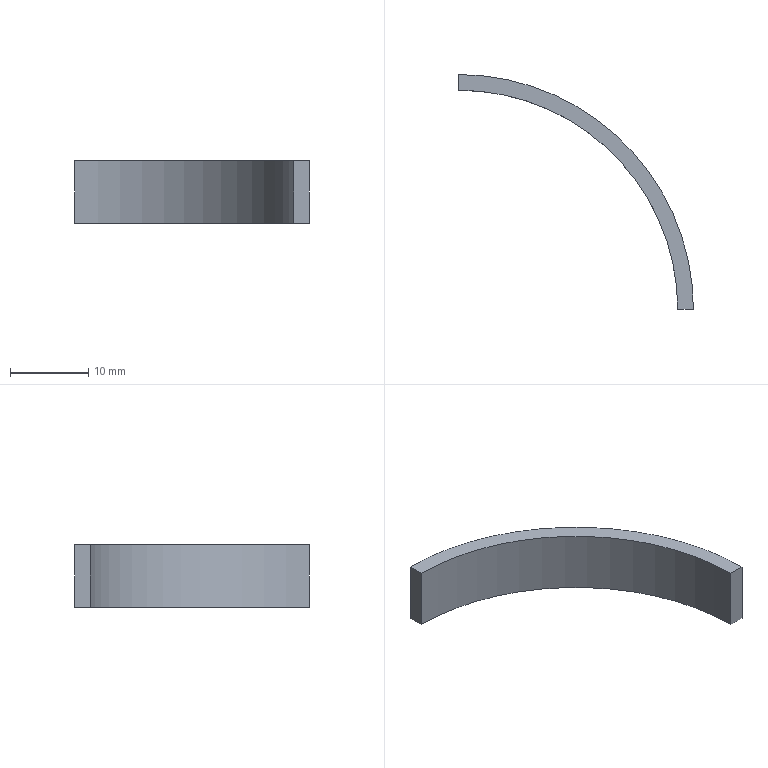Part | STEP file | Oil Pressure Gauge Panel Arc | 1 solid | 6 faces | box 30 x 30 x 8 mm | volume 728.849 mm3 | plane 4 | cylinder 2 | commonest cylinder face diameters 56 x1 60 x1
STEP:
#1=CARTESIAN_POINT('',(-1123.054,332.84,8.));
#2=VERTEX_POINT('',#1);
#3=CARTESIAN_POINT('',(-1093.054,302.84,8.));
#4=VERTEX_POINT('',#3);
#5=CARTESIAN_POINT('',(-1123.054,302.84,8.));
#6=DIRECTION('',(0.,0.,-1.));
#7=DIRECTION('',(-1.,0.,0.));
#8=AXIS2_PLACEMENT_3D('',#5,#6,#7);
#9=CIRCLE('',#8,30.);
#10=EDGE_CURVE('',#2,#4,#9,.T.);
#11=ORIENTED_EDGE('',*,*,#10,.T.);
#12=CARTESIAN_POINT('',(-1093.054,302.84,0.));
#13=VERTEX_POINT('',#12);
#14=CARTESIAN_POINT('',(-1093.054,302.84,8.));
#15=DIRECTION('',(0.,0.,-1.));
#16=VECTOR('',#15,1000.);
#17=LINE('',#14,#16);
#18=EDGE_CURVE('',#4,#13,#17,.T.);
#19=ORIENTED_EDGE('',*,*,#18,.T.);
#20=CARTESIAN_POINT('',(-1123.054,332.84,0.));
#21=VERTEX_POINT('',#20);
#22=CARTESIAN_POINT('',(-1123.054,302.84,0.));
#23=DIRECTION('',(0.,0.,1.));
#24=DIRECTION('',(-1.,0.,0.));
#25=AXIS2_PLACEMENT_3D('',#22,#23,#24);
#26=CIRCLE('',#25,30.);
#27=EDGE_CURVE('',#13,#21,#26,.T.);
#28=ORIENTED_EDGE('',*,*,#27,.T.);
#29=CARTESIAN_POINT('',(-1123.054,332.84,8.));
#30=DIRECTION('',(0.,0.,1.));
#31=VECTOR('',#30,1000.);
#32=LINE('',#29,#31);
#33=EDGE_CURVE('',#21,#2,#32,.T.);
#34=ORIENTED_EDGE('',*,*,#33,.T.);
#35=EDGE_LOOP('',(#11,#19,#28,#34));
#36=FACE_OUTER_BOUND('',#35,.T.);
#37=CARTESIAN_POINT('',(-1123.054,302.84,8.));
#38=DIRECTION('',(0.,0.,-1.));
#39=DIRECTION('',(-1.,0.,0.));
#40=AXIS2_PLACEMENT_3D('',#37,#38,#39);
#41=CYLINDRICAL_SURFACE('',#40,30.);
#42=ADVANCED_FACE('',(#36),#41,.T.);
#43=CARTESIAN_POINT('',(-1095.054,302.84,8.));
#44=VERTEX_POINT('',#43);
#45=CARTESIAN_POINT('',(-1093.054,302.84,8.));
#46=DIRECTION('',(-1.,0.,0.));
#47=VECTOR('',#46,1000.);
#48=LINE('',#45,#47);
#49=EDGE_CURVE('',#4,#44,#48,.T.);
#50=ORIENTED_EDGE('',*,*,#49,.T.);
#51=CARTESIAN_POINT('',(-1095.054,302.84,0.));
#52=VERTEX_POINT('',#51);
#53=CARTESIAN_POINT('',(-1095.054,302.84,8.));
#54=DIRECTION('',(0.,0.,-1.));
#55=VECTOR('',#54,1000.);
#56=LINE('',#53,#55);
#57=EDGE_CURVE('',#44,#52,#56,.T.);
#58=ORIENTED_EDGE('',*,*,#57,.T.);
#59=CARTESIAN_POINT('',(-1093.054,302.84,0.));
#60=DIRECTION('',(1.,0.,0.));
#61=VECTOR('',#60,1000.);
#62=LINE('',#59,#61);
#63=EDGE_CURVE('',#52,#13,#62,.T.);
#64=ORIENTED_EDGE('',*,*,#63,.T.);
#65=ORIENTED_EDGE('',*,*,#18,.F.);
#66=EDGE_LOOP('',(#50,#58,#64,#65));
#67=FACE_OUTER_BOUND('',#66,.T.);
#68=CARTESIAN_POINT('',(-1093.054,302.84,8.));
#69=DIRECTION('',(0.,-1.,0.));
#70=DIRECTION('',(0.,0.,-1.));
#71=AXIS2_PLACEMENT_3D('',#68,#69,#70);
#72=PLANE('',#71);
#73=ADVANCED_FACE('',(#67),#72,.T.);
#74=ORIENTED_EDGE('',*,*,#10,.F.);
#75=CARTESIAN_POINT('',(-1123.054,330.84,8.));
#76=VERTEX_POINT('',#75);
#77=CARTESIAN_POINT('',(-1123.054,302.84,8.));
#78=DIRECTION('',(0.,-1.,0.));
#79=VECTOR('',#78,1000.);
#80=LINE('',#77,#79);
#81=EDGE_CURVE('',#2,#76,#80,.T.);
#82=ORIENTED_EDGE('',*,*,#81,.T.);
#83=CARTESIAN_POINT('',(-1123.054,302.84,8.));
#84=DIRECTION('',(0.,0.,-1.));
#85=DIRECTION('',(-1.,0.,0.));
#86=AXIS2_PLACEMENT_3D('',#83,#84,#85);
#87=CIRCLE('',#86,28.);
#88=EDGE_CURVE('',#76,#44,#87,.T.);
#89=ORIENTED_EDGE('',*,*,#88,.T.);
#90=ORIENTED_EDGE('',*,*,#49,.F.);
#91=EDGE_LOOP('',(#74,#82,#89,#90));
#92=FACE_OUTER_BOUND('',#91,.T.);
#93=CARTESIAN_POINT('',(-1123.054,302.84,8.));
#94=DIRECTION('',(0.,0.,1.));
#95=DIRECTION('',(1.,0.,0.));
#96=AXIS2_PLACEMENT_3D('',#93,#94,#95);
#97=PLANE('',#96);
#98=ADVANCED_FACE('',(#92),#97,.T.);
#99=ORIENTED_EDGE('',*,*,#81,.F.);
#100=ORIENTED_EDGE('',*,*,#33,.F.);
#101=CARTESIAN_POINT('',(-1123.054,330.84,0.));
#102=VERTEX_POINT('',#101);
#103=CARTESIAN_POINT('',(-1123.054,330.84,0.));
#104=DIRECTION('',(0.,-1.,0.));
#105=VECTOR('',#104,1000.);
#106=LINE('',#103,#105);
#107=EDGE_CURVE('',#21,#102,#106,.T.);
#108=ORIENTED_EDGE('',*,*,#107,.T.);
#109=CARTESIAN_POINT('',(-1123.054,330.84,8.));
#110=DIRECTION('',(0.,0.,1.));
#111=VECTOR('',#110,1000.);
#112=LINE('',#109,#111);
#113=EDGE_CURVE('',#102,#76,#112,.T.);
#114=ORIENTED_EDGE('',*,*,#113,.T.);
#115=EDGE_LOOP('',(#99,#100,#108,#114));
#116=FACE_OUTER_BOUND('',#115,.T.);
#117=CARTESIAN_POINT('',(-1123.054,330.84,8.));
#118=DIRECTION('',(-1.,0.,0.));
#119=DIRECTION('',(0.,0.,1.));
#120=AXIS2_PLACEMENT_3D('',#117,#118,#119);
#121=PLANE('',#120);
#122=ADVANCED_FACE('',(#116),#121,.T.);
#123=ORIENTED_EDGE('',*,*,#107,.F.);
#124=ORIENTED_EDGE('',*,*,#27,.F.);
#125=ORIENTED_EDGE('',*,*,#63,.F.);
#126=CARTESIAN_POINT('',(-1123.054,302.84,0.));
#127=DIRECTION('',(0.,0.,-1.));
#128=DIRECTION('',(-1.,0.,0.));
#129=AXIS2_PLACEMENT_3D('',#126,#127,#128);
#130=CIRCLE('',#129,28.);
#131=EDGE_CURVE('',#102,#52,#130,.T.);
#132=ORIENTED_EDGE('',*,*,#131,.F.);
#133=EDGE_LOOP('',(#123,#124,#125,#132));
#134=FACE_OUTER_BOUND('',#133,.T.);
#135=CARTESIAN_POINT('',(-1123.054,302.84,0.));
#136=DIRECTION('',(0.,0.,1.));
#137=DIRECTION('',(1.,0.,0.));
#138=AXIS2_PLACEMENT_3D('',#135,#136,#137);
#139=PLANE('',#138);
#140=ADVANCED_FACE('',(#134),#139,.F.);
#141=ORIENTED_EDGE('',*,*,#57,.F.);
#142=ORIENTED_EDGE('',*,*,#88,.F.);
#143=ORIENTED_EDGE('',*,*,#113,.F.);
#144=ORIENTED_EDGE('',*,*,#131,.T.);
#145=EDGE_LOOP('',(#141,#142,#143,#144));
#146=FACE_OUTER_BOUND('',#145,.T.);
#147=CARTESIAN_POINT('',(-1123.054,302.84,8.));
#148=DIRECTION('',(0.,0.,-1.));
#149=DIRECTION('',(-1.,0.,0.));
#150=AXIS2_PLACEMENT_3D('',#147,#148,#149);
#151=CYLINDRICAL_SURFACE('',#150,28.);
#152=ADVANCED_FACE('',(#146),#151,.F.);
#153=CLOSED_SHELL('',(#42,#73,#98,#122,#140,#152));
#154=MANIFOLD_SOLID_BREP('',#153);
#155=CARTESIAN_POINT('',(0.,0.,0.));
#156=DIRECTION('',(0.,0.,1.));
#157=DIRECTION('',(1.,0.,0.));
#158=AXIS2_PLACEMENT_3D('',#155,#156,#157);
#159=(LENGTH_UNIT()NAMED_UNIT(*)SI_UNIT(.MILLI.,.METRE.));
#160=UNCERTAINTY_MEASURE_WITH_UNIT(LENGTH_MEASURE(0.00001),#159,'','');
#161=(NAMED_UNIT(*)PLANE_ANGLE_UNIT()SI_UNIT($,.RADIAN.));
#162=(NAMED_UNIT(*)SI_UNIT($,.STERADIAN.)SOLID_ANGLE_UNIT());
#163=(GEOMETRIC_REPRESENTATION_CONTEXT(3)GLOBAL_UNCERTAINTY_ASSIGNED_CONTEXT((#160))GLOBAL_UNIT_ASSIGNED_CONTEXT((#159,#161,#162))REPRESENTATION_CONTEXT('',''));
#164=ADVANCED_BREP_SHAPE_REPRESENTATION('',(#154,#158),#163);